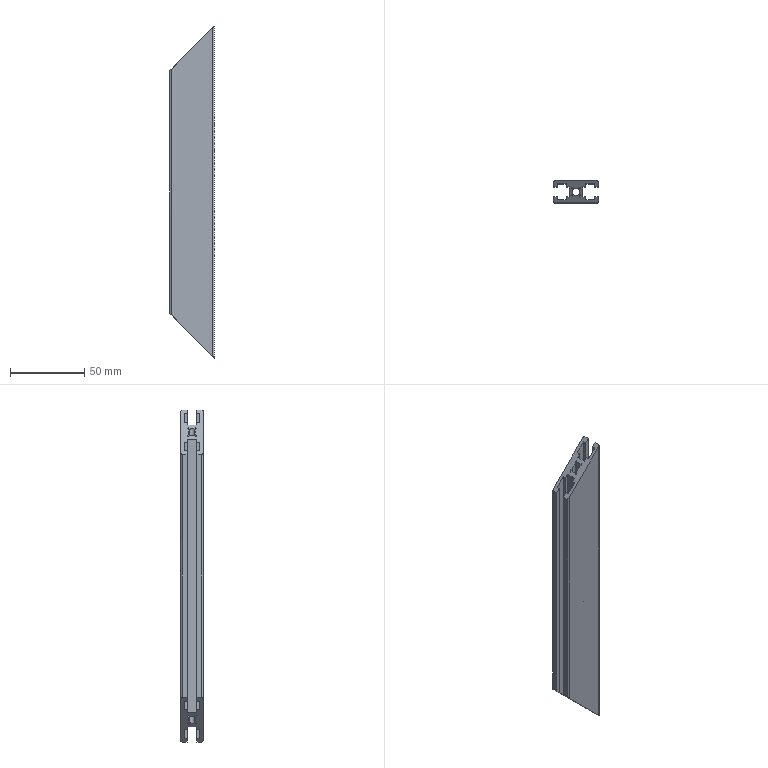Part | NX | features BREP 1 | 1 solid | 95 faces | box 30 x 15 x 223.5 mm | volume 46399 mm3 | plane 46 | cylinder 45 | cone 4 | commonest cylinder face diameters 5 x35 1 x6 2 x4